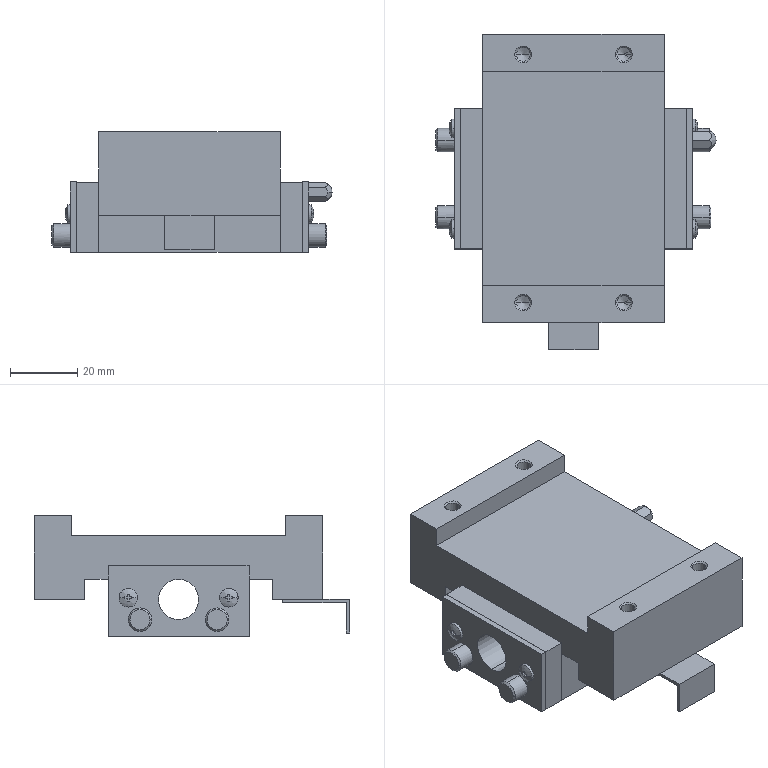Part | STEP file | PRODUCT_ID_2-C-F0-200 | 1 solid | 218 faces | box 83.5 x 94 x 36 mm | volume 123650 mm3 | plane 138 | cylinder 38 | cone 32 | spline 10 | commonest cylinder face diameters 4.134 x8 5.5 x8 7 x8 2.113 x4 3.2 x4 3.22 x4